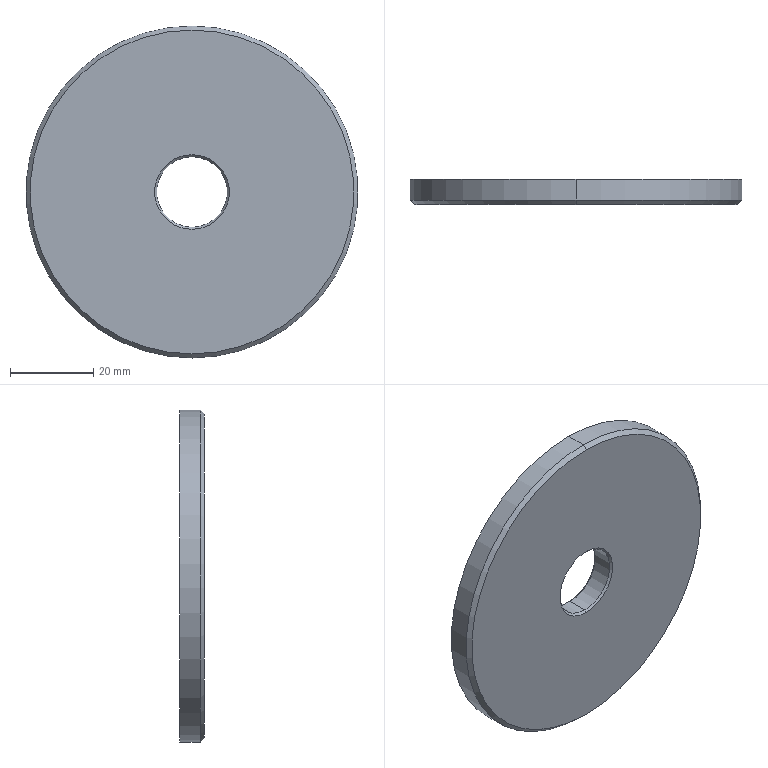Part | SolidWorks | features Chamfer 1, MBimport 1, MoveFace 1 | 1 solid | 12 faces | box 80 x 6.002 x 80 mm | volume 28670 mm3 | cone 6 | cylinder 4 | plane 2 | commonest cylinder face diameters 17 x2 80 x2
STEP:
#1=CARTESIAN_POINT('',(0.,13.392,-9.));
#2=VERTEX_POINT('',#1);
#3=CARTESIAN_POINT('',(0.,13.392,9.));
#4=VERTEX_POINT('',#3);
#5=CARTESIAN_POINT('',(0.,13.392,0.));
#6=DIRECTION('',(0.,-1.,0.));
#7=DIRECTION('',(0.,0.,-1.));
#8=AXIS2_PLACEMENT_3D('',#5,#6,#7);
#9=CIRCLE('',#8,9.);
#10=EDGE_CURVE('',#2,#4,#9,.T.);
#11=ORIENTED_EDGE('',*,*,#10,.T.);
#12=CARTESIAN_POINT('',(0.,13.392,0.));
#13=DIRECTION('',(0.,-1.,0.));
#14=DIRECTION('',(0.,0.,-1.));
#15=AXIS2_PLACEMENT_3D('',#12,#13,#14);
#16=CIRCLE('',#15,9.);
#17=EDGE_CURVE('',#4,#2,#16,.T.);
#18=ORIENTED_EDGE('',*,*,#17,.T.);
#19=EDGE_LOOP('',(#11,#18));
#20=FACE_BOUND('',#19,.T.);
#21=CARTESIAN_POINT('',(0.,13.392,-40.));
#22=VERTEX_POINT('',#21);
#23=CARTESIAN_POINT('',(0.,13.392,40.));
#24=VERTEX_POINT('',#23);
#25=CARTESIAN_POINT('',(0.,13.392,0.));
#26=DIRECTION('',(0.,-1.,0.));
#27=DIRECTION('',(0.,0.,-1.));
#28=AXIS2_PLACEMENT_3D('',#25,#26,#27);
#29=CIRCLE('',#28,40.);
#30=EDGE_CURVE('',#22,#24,#29,.T.);
#31=ORIENTED_EDGE('',*,*,#30,.F.);
#32=CARTESIAN_POINT('',(0.,13.392,0.));
#33=DIRECTION('',(0.,-1.,0.));
#34=DIRECTION('',(0.,0.,-1.));
#35=AXIS2_PLACEMENT_3D('',#32,#33,#34);
#36=CIRCLE('',#35,40.);
#37=EDGE_CURVE('',#24,#22,#36,.T.);
#38=ORIENTED_EDGE('',*,*,#37,.F.);
#39=EDGE_LOOP('',(#31,#38));
#40=FACE_OUTER_BOUND('',#39,.T.);
#41=CARTESIAN_POINT('',(-9.,13.392,0.));
#42=DIRECTION('',(0.,-1.,0.));
#43=DIRECTION('',(0.,0.,-1.));
#44=AXIS2_PLACEMENT_3D('',#41,#42,#43);
#45=PLANE('',#44);
#46=ADVANCED_FACE('',(#20,#40),#45,.F.);
#47=CARTESIAN_POINT('',(0.,7.39,-39.));
#48=VERTEX_POINT('',#47);
#49=CARTESIAN_POINT('',(0.,8.39,-40.));
#50=VERTEX_POINT('',#49);
#51=CARTESIAN_POINT('',(0.,7.39,-39.));
#52=DIRECTION('',(0.,0.7071,-0.7071));
#53=VECTOR('',#52,1000.);
#54=LINE('',#51,#53);
#55=EDGE_CURVE('',#48,#50,#54,.T.);
#56=ORIENTED_EDGE('',*,*,#55,.F.);
#57=CARTESIAN_POINT('',(0.,7.39,39.));
#58=VERTEX_POINT('',#57);
#59=CARTESIAN_POINT('',(0.,7.39,0.));
#60=DIRECTION('',(0.,-1.,0.));
#61=DIRECTION('',(0.,0.,1.));
#62=AXIS2_PLACEMENT_3D('',#59,#60,#61);
#63=CIRCLE('',#62,39.);
#64=EDGE_CURVE('',#58,#48,#63,.T.);
#65=ORIENTED_EDGE('',*,*,#64,.F.);
#66=CARTESIAN_POINT('',(0.,8.39,40.));
#67=VERTEX_POINT('',#66);
#68=CARTESIAN_POINT('',(0.,7.39,39.));
#69=DIRECTION('',(0.,0.7071,0.7071));
#70=VECTOR('',#69,1000.);
#71=LINE('',#68,#70);
#72=EDGE_CURVE('',#58,#67,#71,.T.);
#73=ORIENTED_EDGE('',*,*,#72,.T.);
#74=CARTESIAN_POINT('',(0.,8.39,0.));
#75=DIRECTION('',(0.,1.,0.));
#76=DIRECTION('',(0.,0.,1.));
#77=AXIS2_PLACEMENT_3D('',#74,#75,#76);
#78=CIRCLE('',#77,40.);
#79=EDGE_CURVE('',#50,#67,#78,.T.);
#80=ORIENTED_EDGE('',*,*,#79,.F.);
#81=EDGE_LOOP('',(#56,#65,#73,#80));
#82=FACE_OUTER_BOUND('',#81,.T.);
#83=CARTESIAN_POINT('',(0.,7.39,0.));
#84=DIRECTION('',(0.,1.,0.));
#85=DIRECTION('',(0.,0.,1.));
#86=AXIS2_PLACEMENT_3D('',#83,#84,#85);
#87=CONICAL_SURFACE('',#86,39.,0.7854);
#88=ADVANCED_FACE('',(#82),#87,.T.);
#89=CARTESIAN_POINT('',(0.,12.892,8.5));
#90=VERTEX_POINT('',#89);
#91=CARTESIAN_POINT('',(0.,7.89,8.5));
#92=VERTEX_POINT('',#91);
#93=CARTESIAN_POINT('',(0.,0.,8.5));
#94=DIRECTION('',(0.,-1.,0.));
#95=VECTOR('',#94,1000.);
#96=LINE('',#93,#95);
#97=EDGE_CURVE('',#90,#92,#96,.T.);
#98=ORIENTED_EDGE('',*,*,#97,.F.);
#99=CARTESIAN_POINT('',(0.,12.892,-8.5));
#100=VERTEX_POINT('',#99);
#101=CARTESIAN_POINT('',(0.,12.892,0.));
#102=DIRECTION('',(0.,1.,0.));
#103=DIRECTION('',(0.,0.,-1.));
#104=AXIS2_PLACEMENT_3D('',#101,#102,#103);
#105=CIRCLE('',#104,8.5);
#106=EDGE_CURVE('',#90,#100,#105,.T.);
#107=ORIENTED_EDGE('',*,*,#106,.T.);
#108=CARTESIAN_POINT('',(0.,7.89,-8.5));
#109=VERTEX_POINT('',#108);
#110=CARTESIAN_POINT('',(0.,0.,-8.5));
#111=DIRECTION('',(0.,-1.,0.));
#112=VECTOR('',#111,1000.);
#113=LINE('',#110,#112);
#114=EDGE_CURVE('',#100,#109,#113,.T.);
#115=ORIENTED_EDGE('',*,*,#114,.T.);
#116=CARTESIAN_POINT('',(0.,7.89,0.));
#117=DIRECTION('',(0.,-1.,0.));
#118=DIRECTION('',(0.,0.,-1.));
#119=AXIS2_PLACEMENT_3D('',#116,#117,#118);
#120=CIRCLE('',#119,8.5);
#121=EDGE_CURVE('',#109,#92,#120,.T.);
#122=ORIENTED_EDGE('',*,*,#121,.T.);
#123=EDGE_LOOP('',(#98,#107,#115,#122));
#124=FACE_OUTER_BOUND('',#123,.T.);
#125=CARTESIAN_POINT('',(0.,0.,0.));
#126=DIRECTION('',(0.,-1.,0.));
#127=DIRECTION('',(0.,0.,-1.));
#128=AXIS2_PLACEMENT_3D('',#125,#126,#127);
#129=CYLINDRICAL_SURFACE('',#128,8.5);
#130=ADVANCED_FACE('',(#124),#129,.F.);
#131=CARTESIAN_POINT('',(0.,7.39,9.));
#132=VERTEX_POINT('',#131);
#133=CARTESIAN_POINT('',(0.,7.39,9.));
#134=DIRECTION('',(0.,-0.7071,0.7071));
#135=VECTOR('',#134,1000.);
#136=LINE('',#133,#135);
#137=EDGE_CURVE('',#92,#132,#136,.T.);
#138=ORIENTED_EDGE('',*,*,#137,.F.);
#139=ORIENTED_EDGE('',*,*,#121,.F.);
#140=CARTESIAN_POINT('',(0.,7.39,-9.));
#141=VERTEX_POINT('',#140);
#142=CARTESIAN_POINT('',(0.,7.39,-9.));
#143=DIRECTION('',(0.,-0.7071,-0.7071));
#144=VECTOR('',#143,1000.);
#145=LINE('',#142,#144);
#146=EDGE_CURVE('',#109,#141,#145,.T.);
#147=ORIENTED_EDGE('',*,*,#146,.T.);
#148=CARTESIAN_POINT('',(0.,7.39,0.));
#149=DIRECTION('',(0.,-1.,0.));
#150=DIRECTION('',(0.,0.,-1.));
#151=AXIS2_PLACEMENT_3D('',#148,#149,#150);
#152=CIRCLE('',#151,9.);
#153=EDGE_CURVE('',#141,#132,#152,.T.);
#154=ORIENTED_EDGE('',*,*,#153,.T.);
#155=EDGE_LOOP('',(#138,#139,#147,#154));
#156=FACE_OUTER_BOUND('',#155,.T.);
#157=CARTESIAN_POINT('',(0.,7.39,0.));
#158=DIRECTION('',(0.,-1.,0.));
#159=DIRECTION('',(0.,0.,-1.));
#160=AXIS2_PLACEMENT_3D('',#157,#158,#159);
#161=CONICAL_SURFACE('',#160,9.,0.7854);
#162=ADVANCED_FACE('',(#156),#161,.F.);
#163=ORIENTED_EDGE('',*,*,#153,.F.);
#164=CARTESIAN_POINT('',(0.,7.39,0.));
#165=DIRECTION('',(0.,-1.,0.));
#166=DIRECTION('',(0.,0.,-1.));
#167=AXIS2_PLACEMENT_3D('',#164,#165,#166);
#168=CIRCLE('',#167,9.);
#169=EDGE_CURVE('',#132,#141,#168,.T.);
#170=ORIENTED_EDGE('',*,*,#169,.F.);
#171=EDGE_LOOP('',(#163,#170));
#172=FACE_BOUND('',#171,.T.);
#173=ORIENTED_EDGE('',*,*,#64,.T.);
#174=CARTESIAN_POINT('',(0.,7.39,0.));
#175=DIRECTION('',(0.,-1.,0.));
#176=DIRECTION('',(0.,0.,1.));
#177=AXIS2_PLACEMENT_3D('',#174,#175,#176);
#178=CIRCLE('',#177,39.);
#179=EDGE_CURVE('',#48,#58,#178,.T.);
#180=ORIENTED_EDGE('',*,*,#179,.T.);
#181=EDGE_LOOP('',(#173,#180));
#182=FACE_OUTER_BOUND('',#181,.T.);
#183=CARTESIAN_POINT('',(-40.,7.39,0.));
#184=DIRECTION('',(0.,1.,0.));
#185=DIRECTION('',(1.,0.,0.));
#186=AXIS2_PLACEMENT_3D('',#183,#184,#185);
#187=PLANE('',#186);
#188=ADVANCED_FACE('',(#172,#182),#187,.F.);
#189=CARTESIAN_POINT('',(0.,0.,40.));
#190=DIRECTION('',(0.,-1.,0.));
#191=VECTOR('',#190,1000.);
#192=LINE('',#189,#191);
#193=EDGE_CURVE('',#24,#67,#192,.T.);
#194=ORIENTED_EDGE('',*,*,#193,.F.);
#195=ORIENTED_EDGE('',*,*,#37,.T.);
#196=CARTESIAN_POINT('',(0.,0.,-40.));
#197=DIRECTION('',(0.,-1.,0.));
#198=VECTOR('',#197,1000.);
#199=LINE('',#196,#198);
#200=EDGE_CURVE('',#22,#50,#199,.T.);
#201=ORIENTED_EDGE('',*,*,#200,.T.);
#202=ORIENTED_EDGE('',*,*,#79,.T.);
#203=EDGE_LOOP('',(#194,#195,#201,#202));
#204=FACE_OUTER_BOUND('',#203,.T.);
#205=CARTESIAN_POINT('',(0.,0.,0.));
#206=DIRECTION('',(0.,-1.,0.));
#207=DIRECTION('',(0.,0.,-1.));
#208=AXIS2_PLACEMENT_3D('',#205,#206,#207);
#209=CYLINDRICAL_SURFACE('',#208,40.);
#210=ADVANCED_FACE('',(#204),#209,.T.);
#211=ORIENTED_EDGE('',*,*,#30,.T.);
#212=ORIENTED_EDGE('',*,*,#193,.T.);
#213=CARTESIAN_POINT('',(0.,8.39,0.));
#214=DIRECTION('',(0.,1.,0.));
#215=DIRECTION('',(0.,0.,1.));
#216=AXIS2_PLACEMENT_3D('',#213,#214,#215);
#217=CIRCLE('',#216,40.);
#218=EDGE_CURVE('',#67,#50,#217,.T.);
#219=ORIENTED_EDGE('',*,*,#218,.T.);
#220=ORIENTED_EDGE('',*,*,#200,.F.);
#221=EDGE_LOOP('',(#211,#212,#219,#220));
#222=FACE_OUTER_BOUND('',#221,.T.);
#223=CARTESIAN_POINT('',(0.,0.,0.));
#224=DIRECTION('',(0.,-1.,0.));
#225=DIRECTION('',(0.,0.,-1.));
#226=AXIS2_PLACEMENT_3D('',#223,#224,#225);
#227=CYLINDRICAL_SURFACE('',#226,40.);
#228=ADVANCED_FACE('',(#222),#227,.T.);
#229=CARTESIAN_POINT('',(0.,7.89,0.));
#230=DIRECTION('',(0.,-1.,0.));
#231=DIRECTION('',(0.,0.,-1.));
#232=AXIS2_PLACEMENT_3D('',#229,#230,#231);
#233=CIRCLE('',#232,8.5);
#234=EDGE_CURVE('',#92,#109,#233,.T.);
#235=ORIENTED_EDGE('',*,*,#234,.F.);
#236=ORIENTED_EDGE('',*,*,#137,.T.);
#237=ORIENTED_EDGE('',*,*,#169,.T.);
#238=ORIENTED_EDGE('',*,*,#146,.F.);
#239=EDGE_LOOP('',(#235,#236,#237,#238));
#240=FACE_OUTER_BOUND('',#239,.T.);
#241=CARTESIAN_POINT('',(0.,7.39,0.));
#242=DIRECTION('',(0.,-1.,0.));
#243=DIRECTION('',(0.,0.,-1.));
#244=AXIS2_PLACEMENT_3D('',#241,#242,#243);
#245=CONICAL_SURFACE('',#244,9.,0.7854);
#246=ADVANCED_FACE('',(#240),#245,.F.);
#247=ORIENTED_EDGE('',*,*,#114,.F.);
#248=CARTESIAN_POINT('',(0.,12.892,0.));
#249=DIRECTION('',(0.,1.,0.));
#250=DIRECTION('',(0.,0.,-1.));
#251=AXIS2_PLACEMENT_3D('',#248,#249,#250);
#252=CIRCLE('',#251,8.5);
#253=EDGE_CURVE('',#100,#90,#252,.T.);
#254=ORIENTED_EDGE('',*,*,#253,.T.);
#255=ORIENTED_EDGE('',*,*,#97,.T.);
#256=ORIENTED_EDGE('',*,*,#234,.T.);
#257=EDGE_LOOP('',(#247,#254,#255,#256));
#258=FACE_OUTER_BOUND('',#257,.T.);
#259=CARTESIAN_POINT('',(0.,0.,0.));
#260=DIRECTION('',(0.,-1.,0.));
#261=DIRECTION('',(0.,0.,-1.));
#262=AXIS2_PLACEMENT_3D('',#259,#260,#261);
#263=CYLINDRICAL_SURFACE('',#262,8.5);
#264=ADVANCED_FACE('',(#258),#263,.F.);
#265=ORIENTED_EDGE('',*,*,#179,.F.);
#266=ORIENTED_EDGE('',*,*,#55,.T.);
#267=ORIENTED_EDGE('',*,*,#218,.F.);
#268=ORIENTED_EDGE('',*,*,#72,.F.);
#269=EDGE_LOOP('',(#265,#266,#267,#268));
#270=FACE_OUTER_BOUND('',#269,.T.);
#271=CARTESIAN_POINT('',(0.,7.39,0.));
#272=DIRECTION('',(0.,1.,0.));
#273=DIRECTION('',(0.,0.,1.));
#274=AXIS2_PLACEMENT_3D('',#271,#272,#273);
#275=CONICAL_SURFACE('',#274,39.,0.7854);
#276=ADVANCED_FACE('',(#270),#275,.T.);
#277=CARTESIAN_POINT('',(0.,13.392,9.));
#278=DIRECTION('',(0.,-0.7071,-0.7071));
#279=VECTOR('',#278,1000.);
#280=LINE('',#277,#279);
#281=EDGE_CURVE('',#4,#90,#280,.T.);
#282=ORIENTED_EDGE('',*,*,#281,.F.);
#283=ORIENTED_EDGE('',*,*,#10,.F.);
#284=CARTESIAN_POINT('',(0.,12.892,-8.5));
#285=DIRECTION('',(0.,0.7071,-0.7071));
#286=VECTOR('',#285,1000.);
#287=LINE('',#284,#286);
#288=EDGE_CURVE('',#100,#2,#287,.T.);
#289=ORIENTED_EDGE('',*,*,#288,.F.);
#290=ORIENTED_EDGE('',*,*,#106,.F.);
#291=EDGE_LOOP('',(#282,#283,#289,#290));
#292=FACE_OUTER_BOUND('',#291,.T.);
#293=CARTESIAN_POINT('',(0.,13.392,0.));
#294=DIRECTION('',(0.,1.,0.));
#295=DIRECTION('',(0.,0.,1.));
#296=AXIS2_PLACEMENT_3D('',#293,#294,#295);
#297=CONICAL_SURFACE('',#296,9.,0.7854);
#298=ADVANCED_FACE('',(#292),#297,.F.);
#299=ORIENTED_EDGE('',*,*,#288,.T.);
#300=ORIENTED_EDGE('',*,*,#17,.F.);
#301=ORIENTED_EDGE('',*,*,#281,.T.);
#302=ORIENTED_EDGE('',*,*,#253,.F.);
#303=EDGE_LOOP('',(#299,#300,#301,#302));
#304=FACE_OUTER_BOUND('',#303,.T.);
#305=CARTESIAN_POINT('',(0.,12.892,0.));
#306=DIRECTION('',(0.,1.,0.));
#307=DIRECTION('',(0.,0.,1.));
#308=AXIS2_PLACEMENT_3D('',#305,#306,#307);
#309=CONICAL_SURFACE('',#308,8.5,0.7854);
#310=ADVANCED_FACE('',(#304),#309,.F.);
#311=CLOSED_SHELL('',(#46,#88,#130,#162,#188,#210,#228,#246,#264,#276,#298,#310));
#312=MANIFOLD_SOLID_BREP('',#311);
#313=CARTESIAN_POINT('',(0.,0.,0.));
#314=DIRECTION('',(0.,0.,1.));
#315=DIRECTION('',(1.,0.,0.));
#316=AXIS2_PLACEMENT_3D('',#313,#314,#315);
#317=(LENGTH_UNIT()NAMED_UNIT(*)SI_UNIT(.MILLI.,.METRE.));
#318=UNCERTAINTY_MEASURE_WITH_UNIT(LENGTH_MEASURE(0.00001),#317,'','');
#319=(NAMED_UNIT(*)PLANE_ANGLE_UNIT()SI_UNIT($,.RADIAN.));
#320=(NAMED_UNIT(*)SI_UNIT($,.STERADIAN.)SOLID_ANGLE_UNIT());
#321=(GEOMETRIC_REPRESENTATION_CONTEXT(3)GLOBAL_UNCERTAINTY_ASSIGNED_CONTEXT((#318))GLOBAL_UNIT_ASSIGNED_CONTEXT((#317,#319,#320))REPRESENTATION_CONTEXT('',''));
#322=ADVANCED_BREP_SHAPE_REPRESENTATION('',(#312,#316),#321);